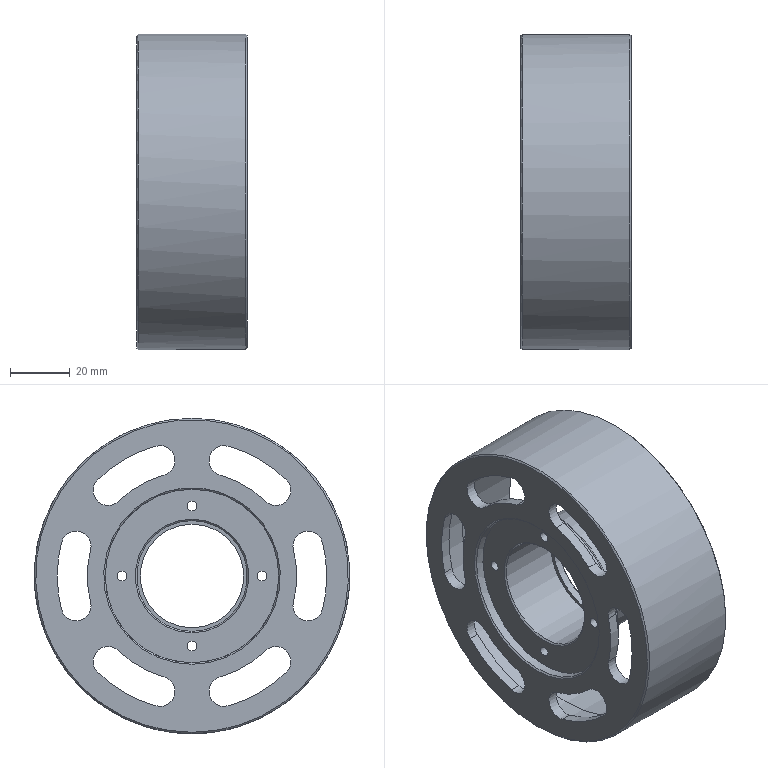Part | NX | features BREP 1 | 1 solid | 54 faces | box 37 x 105.4 x 105.4 mm | volume 69147 mm3 | cylinder 36 | cone 8 | plane 8 | torus 2 | commonest cylinder face diameters 10 x12 70 x6 90 x6 3.3 x4 34.6 x1 37 x1
STEP:
#1=CARTESIAN_POINT('',(6.5,0.,32.));
#2=VERTEX_POINT('',#1);
#3=CARTESIAN_POINT('',(6.5,0.,0.));
#4=DIRECTION('',(-1.,0.,0.));
#5=DIRECTION('',(0.,0.,1.));
#6=AXIS2_PLACEMENT_3D('',#3,#4,#5);
#7=CIRCLE('',#6,32.);
#8=EDGE_CURVE('',#2,#2,#7,.T.);
#9=ORIENTED_EDGE('',*,*,#8,.F.);
#10=EDGE_LOOP('',(#9));
#11=FACE_BOUND('',#10,.T.);
#12=CARTESIAN_POINT('',(8.5,0.,30.));
#13=VERTEX_POINT('',#12);
#14=CARTESIAN_POINT('',(8.5,0.,0.));
#15=DIRECTION('',(1.,0.,0.));
#16=DIRECTION('',(0.,0.,1.));
#17=AXIS2_PLACEMENT_3D('',#14,#15,#16);
#18=CIRCLE('',#17,30.);
#19=EDGE_CURVE('',#13,#13,#18,.T.);
#20=ORIENTED_EDGE('',*,*,#19,.F.);
#21=EDGE_LOOP('',(#20));
#22=FACE_BOUND('',#21,.T.);
#23=CARTESIAN_POINT('',(6.5,0.,0.));
#24=DIRECTION('',(-1.,0.,0.));
#25=DIRECTION('',(0.,0.,1.));
#26=AXIS2_PLACEMENT_3D('',#23,#24,#25);
#27=CONICAL_SURFACE('',#26,32.,0.7854);
#28=ADVANCED_FACE('',(#11,#22),#27,.T.);
#29=CARTESIAN_POINT('',(3.5,9.367,33.723));
#30=VERTEX_POINT('',#29);
#31=CARTESIAN_POINT('',(3.5,12.043,43.359));
#32=VERTEX_POINT('',#31);
#33=CARTESIAN_POINT('',(3.5,10.705,38.541));
#34=DIRECTION('',(-1.,0.,0.));
#35=DIRECTION('',(0.,0.,1.));
#36=AXIS2_PLACEMENT_3D('',#33,#34,#35);
#37=CIRCLE('',#36,5.);
#38=EDGE_CURVE('',#30,#32,#37,.T.);
#39=ORIENTED_EDGE('',*,*,#38,.F.);
#40=CARTESIAN_POINT('',(0.,9.367,33.723));
#41=VERTEX_POINT('',#40);
#42=CARTESIAN_POINT('',(10.,9.367,33.723));
#43=DIRECTION('',(-1.,0.,0.));
#44=VECTOR('',#43,1000.);
#45=LINE('',#42,#44);
#46=EDGE_CURVE('',#30,#41,#45,.T.);
#47=ORIENTED_EDGE('',*,*,#46,.T.);
#48=CARTESIAN_POINT('',(0.,12.043,43.359));
#49=VERTEX_POINT('',#48);
#50=CARTESIAN_POINT('',(0.,10.705,38.541));
#51=DIRECTION('',(-1.,0.,0.));
#52=DIRECTION('',(0.,-0.866,0.5));
#53=AXIS2_PLACEMENT_3D('',#50,#51,#52);
#54=CIRCLE('',#53,5.);
#55=EDGE_CURVE('',#41,#49,#54,.T.);
#56=ORIENTED_EDGE('',*,*,#55,.T.);
#57=CARTESIAN_POINT('',(10.,12.043,43.359));
#58=DIRECTION('',(-1.,0.,0.));
#59=VECTOR('',#58,1000.);
#60=LINE('',#57,#59);
#61=EDGE_CURVE('',#32,#49,#60,.T.);
#62=ORIENTED_EDGE('',*,*,#61,.F.);
#63=EDGE_LOOP('',(#39,#47,#56,#62));
#64=FACE_BOUND('',#63,.T.);
#65=CARTESIAN_POINT('',(10.,10.705,38.541));
#66=DIRECTION('',(-1.,0.,0.));
#67=DIRECTION('',(0.,0.,1.));
#68=AXIS2_PLACEMENT_3D('',#65,#66,#67);
#69=CYLINDRICAL_SURFACE('',#68,5.);
#70=ADVANCED_FACE('',(#64),#69,.F.);
#71=CARTESIAN_POINT('',(3.5,-12.043,43.359));
#72=VERTEX_POINT('',#71);
#73=CARTESIAN_POINT('',(3.5,-9.367,33.723));
#74=VERTEX_POINT('',#73);
#75=CARTESIAN_POINT('',(3.5,-10.705,38.541));
#76=DIRECTION('',(-1.,0.,0.));
#77=DIRECTION('',(0.,0.,1.));
#78=AXIS2_PLACEMENT_3D('',#75,#76,#77);
#79=CIRCLE('',#78,5.);
#80=EDGE_CURVE('',#72,#74,#79,.T.);
#81=ORIENTED_EDGE('',*,*,#80,.F.);
#82=CARTESIAN_POINT('',(0.,-12.043,43.359));
#83=VERTEX_POINT('',#82);
#84=CARTESIAN_POINT('',(10.,-12.043,43.359));
#85=DIRECTION('',(-1.,0.,0.));
#86=VECTOR('',#85,1000.);
#87=LINE('',#84,#86);
#88=EDGE_CURVE('',#72,#83,#87,.T.);
#89=ORIENTED_EDGE('',*,*,#88,.T.);
#90=CARTESIAN_POINT('',(0.,-9.367,33.723));
#91=VERTEX_POINT('',#90);
#92=CARTESIAN_POINT('',(0.,-10.705,38.541));
#93=DIRECTION('',(-1.,0.,0.));
#94=DIRECTION('',(0.,-0.866,-0.5));
#95=AXIS2_PLACEMENT_3D('',#92,#93,#94);
#96=CIRCLE('',#95,5.);
#97=EDGE_CURVE('',#83,#91,#96,.T.);
#98=ORIENTED_EDGE('',*,*,#97,.T.);
#99=CARTESIAN_POINT('',(10.,-9.367,33.723));
#100=DIRECTION('',(-1.,0.,0.));
#101=VECTOR('',#100,1000.);
#102=LINE('',#99,#101);
#103=EDGE_CURVE('',#74,#91,#102,.T.);
#104=ORIENTED_EDGE('',*,*,#103,.F.);
#105=EDGE_LOOP('',(#81,#89,#98,#104));
#106=FACE_BOUND('',#105,.T.);
#107=CARTESIAN_POINT('',(10.,-10.705,38.541));
#108=DIRECTION('',(-1.,0.,0.));
#109=DIRECTION('',(0.,0.,1.));
#110=AXIS2_PLACEMENT_3D('',#107,#108,#109);
#111=CYLINDRICAL_SURFACE('',#110,5.);
#112=ADVANCED_FACE('',(#106),#111,.F.);
#113=CARTESIAN_POINT('',(3.5,-43.571,11.25));
#114=VERTEX_POINT('',#113);
#115=CARTESIAN_POINT('',(3.5,-33.889,8.75));
#116=VERTEX_POINT('',#115);
#117=CARTESIAN_POINT('',(3.5,-38.73,10.));
#118=DIRECTION('',(-1.,0.,0.));
#119=DIRECTION('',(0.,0.,1.));
#120=AXIS2_PLACEMENT_3D('',#117,#118,#119);
#121=CIRCLE('',#120,5.);
#122=EDGE_CURVE('',#114,#116,#121,.T.);
#123=ORIENTED_EDGE('',*,*,#122,.F.);
#124=CARTESIAN_POINT('',(0.,-43.571,11.25));
#125=VERTEX_POINT('',#124);
#126=CARTESIAN_POINT('',(10.,-43.571,11.25));
#127=DIRECTION('',(-1.,0.,0.));
#128=VECTOR('',#127,1000.);
#129=LINE('',#126,#128);
#130=EDGE_CURVE('',#114,#125,#129,.T.);
#131=ORIENTED_EDGE('',*,*,#130,.T.);
#132=CARTESIAN_POINT('',(0.,-33.889,8.75));
#133=VERTEX_POINT('',#132);
#134=CARTESIAN_POINT('',(0.,-38.73,10.));
#135=DIRECTION('',(-1.,0.,0.));
#136=DIRECTION('',(0.,0.,-1.));
#137=AXIS2_PLACEMENT_3D('',#134,#135,#136);
#138=CIRCLE('',#137,5.);
#139=EDGE_CURVE('',#125,#133,#138,.T.);
#140=ORIENTED_EDGE('',*,*,#139,.T.);
#141=CARTESIAN_POINT('',(10.,-33.889,8.75));
#142=DIRECTION('',(-1.,0.,0.));
#143=VECTOR('',#142,1000.);
#144=LINE('',#141,#143);
#145=EDGE_CURVE('',#116,#133,#144,.T.);
#146=ORIENTED_EDGE('',*,*,#145,.F.);
#147=EDGE_LOOP('',(#123,#131,#140,#146));
#148=FACE_BOUND('',#147,.T.);
#149=CARTESIAN_POINT('',(10.,-38.73,10.));
#150=DIRECTION('',(-1.,0.,0.));
#151=DIRECTION('',(0.,0.,1.));
#152=AXIS2_PLACEMENT_3D('',#149,#150,#151);
#153=CYLINDRICAL_SURFACE('',#152,5.);
#154=ADVANCED_FACE('',(#148),#153,.F.);
#155=CARTESIAN_POINT('',(3.5,-31.528,-32.109));
#156=VERTEX_POINT('',#155);
#157=CARTESIAN_POINT('',(3.5,-24.522,-24.973));
#158=VERTEX_POINT('',#157);
#159=CARTESIAN_POINT('',(3.5,-28.025,-28.541));
#160=DIRECTION('',(-1.,0.,0.));
#161=DIRECTION('',(0.,0.,1.));
#162=AXIS2_PLACEMENT_3D('',#159,#160,#161);
#163=CIRCLE('',#162,5.);
#164=EDGE_CURVE('',#156,#158,#163,.T.);
#165=ORIENTED_EDGE('',*,*,#164,.F.);
#166=CARTESIAN_POINT('',(0.,-31.528,-32.109));
#167=VERTEX_POINT('',#166);
#168=CARTESIAN_POINT('',(10.,-31.528,-32.109));
#169=DIRECTION('',(-1.,0.,0.));
#170=VECTOR('',#169,1000.);
#171=LINE('',#168,#170);
#172=EDGE_CURVE('',#156,#167,#171,.T.);
#173=ORIENTED_EDGE('',*,*,#172,.T.);
#174=CARTESIAN_POINT('',(0.,-24.522,-24.973));
#175=VERTEX_POINT('',#174);
#176=CARTESIAN_POINT('',(0.,-28.025,-28.541));
#177=DIRECTION('',(-1.,0.,0.));
#178=DIRECTION('',(0.,0.866,-0.5));
#179=AXIS2_PLACEMENT_3D('',#176,#177,#178);
#180=CIRCLE('',#179,5.);
#181=EDGE_CURVE('',#167,#175,#180,.T.);
#182=ORIENTED_EDGE('',*,*,#181,.T.);
#183=CARTESIAN_POINT('',(10.,-24.522,-24.973));
#184=DIRECTION('',(-1.,0.,0.));
#185=VECTOR('',#184,1000.);
#186=LINE('',#183,#185);
#187=EDGE_CURVE('',#158,#175,#186,.T.);
#188=ORIENTED_EDGE('',*,*,#187,.F.);
#189=EDGE_LOOP('',(#165,#173,#182,#188));
#190=FACE_BOUND('',#189,.T.);
#191=CARTESIAN_POINT('',(10.,-28.025,-28.541));
#192=DIRECTION('',(-1.,0.,0.));
#193=DIRECTION('',(0.,0.,1.));
#194=AXIS2_PLACEMENT_3D('',#191,#192,#193);
#195=CYLINDRICAL_SURFACE('',#194,5.);
#196=ADVANCED_FACE('',(#190),#195,.F.);
#197=CARTESIAN_POINT('',(3.5,24.522,-24.973));
#198=VERTEX_POINT('',#197);
#199=CARTESIAN_POINT('',(3.5,31.528,-32.109));
#200=VERTEX_POINT('',#199);
#201=CARTESIAN_POINT('',(3.5,28.025,-28.541));
#202=DIRECTION('',(-1.,0.,0.));
#203=DIRECTION('',(0.,0.,1.));
#204=AXIS2_PLACEMENT_3D('',#201,#202,#203);
#205=CIRCLE('',#204,5.);
#206=EDGE_CURVE('',#198,#200,#205,.T.);
#207=ORIENTED_EDGE('',*,*,#206,.F.);
#208=CARTESIAN_POINT('',(0.,24.522,-24.973));
#209=VERTEX_POINT('',#208);
#210=CARTESIAN_POINT('',(10.,24.522,-24.973));
#211=DIRECTION('',(-1.,0.,0.));
#212=VECTOR('',#211,1000.);
#213=LINE('',#210,#212);
#214=EDGE_CURVE('',#198,#209,#213,.T.);
#215=ORIENTED_EDGE('',*,*,#214,.T.);
#216=CARTESIAN_POINT('',(0.,31.528,-32.109));
#217=VERTEX_POINT('',#216);
#218=CARTESIAN_POINT('',(0.,28.025,-28.541));
#219=DIRECTION('',(-1.,0.,0.));
#220=DIRECTION('',(0.,0.866,0.5));
#221=AXIS2_PLACEMENT_3D('',#218,#219,#220);
#222=CIRCLE('',#221,5.);
#223=EDGE_CURVE('',#209,#217,#222,.T.);
#224=ORIENTED_EDGE('',*,*,#223,.T.);
#225=CARTESIAN_POINT('',(10.,31.528,-32.109));
#226=DIRECTION('',(-1.,0.,0.));
#227=VECTOR('',#226,1000.);
#228=LINE('',#225,#227);
#229=EDGE_CURVE('',#200,#217,#228,.T.);
#230=ORIENTED_EDGE('',*,*,#229,.F.);
#231=EDGE_LOOP('',(#207,#215,#224,#230));
#232=FACE_BOUND('',#231,.T.);
#233=CARTESIAN_POINT('',(10.,28.025,-28.541));
#234=DIRECTION('',(-1.,0.,0.));
#235=DIRECTION('',(0.,0.,1.));
#236=AXIS2_PLACEMENT_3D('',#233,#234,#235);
#237=CYLINDRICAL_SURFACE('',#236,5.);
#238=ADVANCED_FACE('',(#232),#237,.F.);
#239=CARTESIAN_POINT('',(3.5,33.889,8.75));
#240=VERTEX_POINT('',#239);
#241=CARTESIAN_POINT('',(3.5,43.571,11.25));
#242=VERTEX_POINT('',#241);
#243=CARTESIAN_POINT('',(3.5,38.73,10.));
#244=DIRECTION('',(-1.,0.,0.));
#245=DIRECTION('',(0.,0.,1.));
#246=AXIS2_PLACEMENT_3D('',#243,#244,#245);
#247=CIRCLE('',#246,5.);
#248=EDGE_CURVE('',#240,#242,#247,.T.);
#249=ORIENTED_EDGE('',*,*,#248,.F.);
#250=CARTESIAN_POINT('',(0.,33.889,8.75));
#251=VERTEX_POINT('',#250);
#252=CARTESIAN_POINT('',(10.,33.889,8.75));
#253=DIRECTION('',(-1.,0.,0.));
#254=VECTOR('',#253,1000.);
#255=LINE('',#252,#254);
#256=EDGE_CURVE('',#240,#251,#255,.T.);
#257=ORIENTED_EDGE('',*,*,#256,.T.);
#258=CARTESIAN_POINT('',(0.,43.571,11.25));
#259=VERTEX_POINT('',#258);
#260=CARTESIAN_POINT('',(0.,38.73,10.));
#261=DIRECTION('',(-1.,0.,0.));
#262=DIRECTION('',(0.,0.,1.));
#263=AXIS2_PLACEMENT_3D('',#260,#261,#262);
#264=CIRCLE('',#263,5.);
#265=EDGE_CURVE('',#251,#259,#264,.T.);
#266=ORIENTED_EDGE('',*,*,#265,.T.);
#267=CARTESIAN_POINT('',(10.,43.571,11.25));
#268=DIRECTION('',(-1.,0.,0.));
#269=VECTOR('',#268,1000.);
#270=LINE('',#267,#269);
#271=EDGE_CURVE('',#242,#259,#270,.T.);
#272=ORIENTED_EDGE('',*,*,#271,.F.);
#273=EDGE_LOOP('',(#249,#257,#266,#272));
#274=FACE_BOUND('',#273,.T.);
#275=CARTESIAN_POINT('',(10.,38.73,10.));
#276=DIRECTION('',(-1.,0.,0.));
#277=DIRECTION('',(0.,0.,1.));
#278=AXIS2_PLACEMENT_3D('',#275,#276,#277);
#279=CYLINDRICAL_SURFACE('',#278,5.);
#280=ADVANCED_FACE('',(#274),#279,.F.);
#281=CARTESIAN_POINT('',(3.5,23.4,1.65));
#282=VERTEX_POINT('',#281);
#283=CARTESIAN_POINT('',(3.5,23.4,0.));
#284=DIRECTION('',(-1.,0.,0.));
#285=DIRECTION('',(0.,0.,1.));
#286=AXIS2_PLACEMENT_3D('',#283,#284,#285);
#287=CIRCLE('',#286,1.65);
#288=EDGE_CURVE('',#282,#282,#287,.T.);
#289=ORIENTED_EDGE('',*,*,#288,.T.);
#290=EDGE_LOOP('',(#289));
#291=FACE_BOUND('',#290,.T.);
#292=CARTESIAN_POINT('',(8.5,23.4,1.65));
#293=VERTEX_POINT('',#292);
#294=CARTESIAN_POINT('',(8.5,23.4,0.));
#295=DIRECTION('',(-1.,0.,0.));
#296=DIRECTION('',(0.,0.,1.));
#297=AXIS2_PLACEMENT_3D('',#294,#295,#296);
#298=CIRCLE('',#297,1.65);
#299=EDGE_CURVE('',#293,#293,#298,.T.);
#300=ORIENTED_EDGE('',*,*,#299,.F.);
#301=EDGE_LOOP('',(#300));
#302=FACE_BOUND('',#301,.T.);
#303=CARTESIAN_POINT('',(3.5,23.4,0.));
#304=DIRECTION('',(-1.,0.,0.));
#305=DIRECTION('',(0.,0.,1.));
#306=AXIS2_PLACEMENT_3D('',#303,#304,#305);
#307=CYLINDRICAL_SURFACE('',#306,1.65);
#308=ADVANCED_FACE('',(#291,#302),#307,.F.);
#309=CARTESIAN_POINT('',(3.5,0.,25.05));
#310=VERTEX_POINT('',#309);
#311=CARTESIAN_POINT('',(3.5,0.,23.4));
#312=DIRECTION('',(-1.,0.,0.));
#313=DIRECTION('',(0.,0.,1.));
#314=AXIS2_PLACEMENT_3D('',#311,#312,#313);
#315=CIRCLE('',#314,1.65);
#316=EDGE_CURVE('',#310,#310,#315,.T.);
#317=ORIENTED_EDGE('',*,*,#316,.T.);
#318=EDGE_LOOP('',(#317));
#319=FACE_BOUND('',#318,.T.);
#320=CARTESIAN_POINT('',(8.5,0.,25.05));
#321=VERTEX_POINT('',#320);
#322=CARTESIAN_POINT('',(8.5,0.,23.4));
#323=DIRECTION('',(-1.,0.,0.));
#324=DIRECTION('',(0.,0.,1.));
#325=AXIS2_PLACEMENT_3D('',#322,#323,#324);
#326=CIRCLE('',#325,1.65);
#327=EDGE_CURVE('',#321,#321,#326,.T.);
#328=ORIENTED_EDGE('',*,*,#327,.F.);
#329=EDGE_LOOP('',(#328));
#330=FACE_BOUND('',#329,.T.);
#331=CARTESIAN_POINT('',(3.5,0.,23.4));
#332=DIRECTION('',(-1.,0.,0.));
#333=DIRECTION('',(0.,0.,1.));
#334=AXIS2_PLACEMENT_3D('',#331,#332,#333);
#335=CYLINDRICAL_SURFACE('',#334,1.65);
#336=ADVANCED_FACE('',(#319,#330),#335,.F.);
#337=CARTESIAN_POINT('',(3.5,-23.4,1.65));
#338=VERTEX_POINT('',#337);
#339=CARTESIAN_POINT('',(3.5,-23.4,0.));
#340=DIRECTION('',(-1.,0.,0.));
#341=DIRECTION('',(0.,0.,1.));
#342=AXIS2_PLACEMENT_3D('',#339,#340,#341);
#343=CIRCLE('',#342,1.65);
#344=EDGE_CURVE('',#338,#338,#343,.T.);
#345=ORIENTED_EDGE('',*,*,#344,.T.);
#346=EDGE_LOOP('',(#345));
#347=FACE_BOUND('',#346,.T.);
#348=CARTESIAN_POINT('',(8.5,-23.4,1.65));
#349=VERTEX_POINT('',#348);
#350=CARTESIAN_POINT('',(8.5,-23.4,0.));
#351=DIRECTION('',(-1.,0.,0.));
#352=DIRECTION('',(0.,0.,1.));
#353=AXIS2_PLACEMENT_3D('',#350,#351,#352);
#354=CIRCLE('',#353,1.65);
#355=EDGE_CURVE('',#349,#349,#354,.T.);
#356=ORIENTED_EDGE('',*,*,#355,.F.);
#357=EDGE_LOOP('',(#356));
#358=FACE_BOUND('',#357,.T.);
#359=CARTESIAN_POINT('',(3.5,-23.4,0.));
#360=DIRECTION('',(-1.,0.,0.));
#361=DIRECTION('',(0.,0.,1.));
#362=AXIS2_PLACEMENT_3D('',#359,#360,#361);
#363=CYLINDRICAL_SURFACE('',#362,1.65);
#364=ADVANCED_FACE('',(#347,#358),#363,.F.);
#365=CARTESIAN_POINT('',(3.5,0.,-21.75));
#366=VERTEX_POINT('',#365);
#367=CARTESIAN_POINT('',(3.5,0.,-23.4));
#368=DIRECTION('',(-1.,0.,0.));
#369=DIRECTION('',(0.,0.,1.));
#370=AXIS2_PLACEMENT_3D('',#367,#368,#369);
#371=CIRCLE('',#370,1.65);
#372=EDGE_CURVE('',#366,#366,#371,.T.);
#373=ORIENTED_EDGE('',*,*,#372,.T.);
#374=EDGE_LOOP('',(#373));
#375=FACE_BOUND('',#374,.T.);
#376=CARTESIAN_POINT('',(8.5,0.,-21.75));
#377=VERTEX_POINT('',#376);
#378=CARTESIAN_POINT('',(8.5,0.,-23.4));
#379=DIRECTION('',(-1.,0.,0.));
#380=DIRECTION('',(0.,0.,1.));
#381=AXIS2_PLACEMENT_3D('',#378,#379,#380);
#382=CIRCLE('',#381,1.65);
#383=EDGE_CURVE('',#377,#377,#382,.T.);
#384=ORIENTED_EDGE('',*,*,#383,.F.);
#385=EDGE_LOOP('',(#384));
#386=FACE_BOUND('',#385,.T.);
#387=CARTESIAN_POINT('',(3.5,0.,-23.4));
#388=DIRECTION('',(-1.,0.,0.));
#389=DIRECTION('',(0.,0.,1.));
#390=AXIS2_PLACEMENT_3D('',#387,#388,#389);
#391=CYLINDRICAL_SURFACE('',#390,1.65);
#392=ADVANCED_FACE('',(#375,#386),#391,.F.);
#393=CARTESIAN_POINT('',(28.,0.,17.8));
#394=VERTEX_POINT('',#393);
#395=CARTESIAN_POINT('',(28.,0.,0.));
#396=DIRECTION('',(-1.,0.,0.));
#397=DIRECTION('',(0.,0.,1.));
#398=AXIS2_PLACEMENT_3D('',#395,#396,#397);
#399=CIRCLE('',#398,17.8);
#400=EDGE_CURVE('',#394,#394,#399,.T.);
#401=ORIENTED_EDGE('',*,*,#400,.F.);
#402=EDGE_LOOP('',(#401));
#403=FACE_BOUND('',#402,.T.);
#404=CARTESIAN_POINT('',(27.5,0.,17.3));
#405=VERTEX_POINT('',#404);
#406=CARTESIAN_POINT('',(27.5,0.,0.));
#407=DIRECTION('',(1.,0.,0.));
#408=DIRECTION('',(0.,0.,1.));
#409=AXIS2_PLACEMENT_3D('',#406,#407,#408);
#410=CIRCLE('',#409,17.3);
#411=EDGE_CURVE('',#405,#405,#410,.T.);
#412=ORIENTED_EDGE('',*,*,#411,.F.);
#413=EDGE_LOOP('',(#412));
#414=FACE_BOUND('',#413,.T.);
#415=CARTESIAN_POINT('',(28.,0.,0.));
#416=DIRECTION('',(1.,0.,0.));
#417=DIRECTION('',(0.,0.,-1.));
#418=AXIS2_PLACEMENT_3D('',#415,#416,#417);
#419=CONICAL_SURFACE('',#418,17.8,0.7854);
#420=ADVANCED_FACE('',(#403,#414),#419,.F.);
#421=CARTESIAN_POINT('',(0.5,0.,-52.7));
#422=VERTEX_POINT('',#421);
#423=CARTESIAN_POINT('',(0.5,0.,0.));
#424=DIRECTION('',(1.,0.,0.));
#425=DIRECTION('',(0.,0.,-1.));
#426=AXIS2_PLACEMENT_3D('',#423,#424,#425);
#427=CIRCLE('',#426,52.7);
#428=EDGE_CURVE('',#422,#422,#427,.T.);
#429=ORIENTED_EDGE('',*,*,#428,.F.);
#430=EDGE_LOOP('',(#429));
#431=FACE_BOUND('',#430,.T.);
#432=CARTESIAN_POINT('',(0.,0.,-52.2));
#433=VERTEX_POINT('',#432);
#434=CARTESIAN_POINT('',(0.,0.,0.));
#435=DIRECTION('',(-1.,0.,0.));
#436=DIRECTION('',(0.,0.,-1.));
#437=AXIS2_PLACEMENT_3D('',#434,#435,#436);
#438=CIRCLE('',#437,52.2);
#439=EDGE_CURVE('',#433,#433,#438,.T.);
#440=ORIENTED_EDGE('',*,*,#439,.F.);
#441=EDGE_LOOP('',(#440));
#442=FACE_BOUND('',#441,.T.);
#443=CARTESIAN_POINT('',(0.,0.,0.));
#444=DIRECTION('',(1.,0.,0.));
#445=DIRECTION('',(0.,0.,-1.));
#446=AXIS2_PLACEMENT_3D('',#443,#444,#445);
#447=CONICAL_SURFACE('',#446,52.2,0.7854);
#448=ADVANCED_FACE('',(#431,#442),#447,.T.);
#449=CARTESIAN_POINT('',(0.,0.,-29.5));
#450=VERTEX_POINT('',#449);
#451=CARTESIAN_POINT('',(0.,0.,0.));
#452=DIRECTION('',(1.,0.,0.));
#453=DIRECTION('',(0.,0.,-1.));
#454=AXIS2_PLACEMENT_3D('',#451,#452,#453);
#455=CIRCLE('',#454,29.5);
#456=EDGE_CURVE('',#450,#450,#455,.T.);
#457=ORIENTED_EDGE('',*,*,#456,.F.);
#458=EDGE_LOOP('',(#457));
#459=FACE_BOUND('',#458,.T.);
#460=CARTESIAN_POINT('',(0.5,0.,-29.));
#461=VERTEX_POINT('',#460);
#462=CARTESIAN_POINT('',(0.5,0.,0.));
#463=DIRECTION('',(-1.,0.,0.));
#464=DIRECTION('',(0.,0.,-1.));
#465=AXIS2_PLACEMENT_3D('',#462,#463,#464);
#466=CIRCLE('',#465,29.);
#467=EDGE_CURVE('',#461,#461,#466,.T.);
#468=ORIENTED_EDGE('',*,*,#467,.F.);
#469=EDGE_LOOP('',(#468));
#470=FACE_BOUND('',#469,.T.);
#471=CARTESIAN_POINT('',(0.5,0.,0.));
#472=DIRECTION('',(-1.,0.,0.));
#473=DIRECTION('',(0.,0.,1.));
#474=AXIS2_PLACEMENT_3D('',#471,#472,#473);
#475=CONICAL_SURFACE('',#474,29.,0.7854);
#476=ADVANCED_FACE('',(#459,#470),#475,.F.);
#477=CARTESIAN_POINT('',(3.5,0.,-19.));
#478=VERTEX_POINT('',#477);
#479=CARTESIAN_POINT('',(3.5,0.,0.));
#480=DIRECTION('',(1.,0.,0.));
#481=DIRECTION('',(0.,0.,-1.));
#482=AXIS2_PLACEMENT_3D('',#479,#480,#481);
#483=CIRCLE('',#482,19.);
#484=EDGE_CURVE('',#478,#478,#483,.T.);
#485=ORIENTED_EDGE('',*,*,#484,.F.);
#486=EDGE_LOOP('',(#485));
#487=FACE_BOUND('',#486,.T.);
#488=CARTESIAN_POINT('',(4.,0.,-18.5));
#489=VERTEX_POINT('',#488);
#490=CARTESIAN_POINT('',(4.,0.,0.));
#491=DIRECTION('',(-1.,0.,0.));
#492=DIRECTION('',(0.,0.,-1.));
#493=AXIS2_PLACEMENT_3D('',#490,#491,#492);
#494=CIRCLE('',#493,18.5);
#495=EDGE_CURVE('',#489,#489,#494,.T.);
#496=ORIENTED_EDGE('',*,*,#495,.F.);
#497=EDGE_LOOP('',(#496));
#498=FACE_BOUND('',#497,.T.);
#499=CARTESIAN_POINT('',(4.,0.,0.));
#500=DIRECTION('',(-1.,0.,0.));
#501=DIRECTION('',(0.,0.,1.));
#502=AXIS2_PLACEMENT_3D('',#499,#500,#501);
#503=CONICAL_SURFACE('',#502,18.5,0.7854);
#504=ADVANCED_FACE('',(#487,#498),#503,.F.);
#505=CARTESIAN_POINT('',(27.5,0.,21.25));
#506=VERTEX_POINT('',#505);
#507=CARTESIAN_POINT('',(27.5,0.,0.));
#508=DIRECTION('',(-1.,0.,0.));
#509=DIRECTION('',(0.,0.,1.));
#510=AXIS2_PLACEMENT_3D('',#507,#508,#509);
#511=CIRCLE('',#510,21.25);
#512=EDGE_CURVE('',#506,#506,#511,.T.);
#513=ORIENTED_EDGE('',*,*,#512,.F.);
#514=EDGE_LOOP('',(#513));
#515=FACE_BOUND('',#514,.T.);
#516=CARTESIAN_POINT('',(28.,0.,20.75));
#517=VERTEX_POINT('',#516);
#518=CARTESIAN_POINT('',(28.,0.,0.));
#519=DIRECTION('',(1.,0.,0.));
#520=DIRECTION('',(0.,0.,1.));
#521=AXIS2_PLACEMENT_3D('',#518,#519,#520);
#522=CIRCLE('',#521,20.75);
#523=EDGE_CURVE('',#517,#517,#522,.T.);
#524=ORIENTED_EDGE('',*,*,#523,.F.);
#525=EDGE_LOOP('',(#524));
#526=FACE_BOUND('',#525,.T.);
#527=CARTESIAN_POINT('',(27.5,0.,0.));
#528=DIRECTION('',(-1.,0.,0.));
#529=DIRECTION('',(0.,0.,1.));
#530=AXIS2_PLACEMENT_3D('',#527,#528,#529);
#531=CONICAL_SURFACE('',#530,21.25,0.7854);
#532=ADVANCED_FACE('',(#515,#526),#531,.T.);
#533=CARTESIAN_POINT('',(37.,0.,49.9));
#534=VERTEX_POINT('',#533);
#535=CARTESIAN_POINT('',(37.,0.,0.));
#536=DIRECTION('',(-1.,0.,0.));
#537=DIRECTION('',(0.,0.,1.));
#538=AXIS2_PLACEMENT_3D('',#535,#536,#537);
#539=CIRCLE('',#538,49.9);
#540=EDGE_CURVE('',#534,#534,#539,.T.);
#541=ORIENTED_EDGE('',*,*,#540,.F.);
#542=EDGE_LOOP('',(#541));
#543=FACE_BOUND('',#542,.T.);
#544=CARTESIAN_POINT('',(36.5,0.,49.4));
#545=VERTEX_POINT('',#544);
#546=CARTESIAN_POINT('',(36.5,0.,0.));
#547=DIRECTION('',(1.,0.,0.));
#548=DIRECTION('',(0.,0.,1.));
#549=AXIS2_PLACEMENT_3D('',#546,#547,#548);
#550=CIRCLE('',#549,49.4);
#551=EDGE_CURVE('',#545,#545,#550,.T.);
#552=ORIENTED_EDGE('',*,*,#551,.F.);
#553=EDGE_LOOP('',(#552));
#554=FACE_BOUND('',#553,.T.);
#555=CARTESIAN_POINT('',(37.,0.,0.));
#556=DIRECTION('',(1.,0.,0.));
#557=DIRECTION('',(0.,0.,-1.));
#558=AXIS2_PLACEMENT_3D('',#555,#556,#557);
#559=CONICAL_SURFACE('',#558,49.9,0.7854);
#560=ADVANCED_FACE('',(#543,#554),#559,.F.);
#561=CARTESIAN_POINT('',(36.5,0.,52.7));
#562=VERTEX_POINT('',#561);
#563=CARTESIAN_POINT('',(36.5,0.,0.));
#564=DIRECTION('',(-1.,0.,0.));
#565=DIRECTION('',(0.,0.,1.));
#566=AXIS2_PLACEMENT_3D('',#563,#564,#565);
#567=CIRCLE('',#566,52.7);
#568=EDGE_CURVE('',#562,#562,#567,.T.);
#569=ORIENTED_EDGE('',*,*,#568,.F.);
#570=EDGE_LOOP('',(#569));
#571=FACE_BOUND('',#570,.T.);
#572=CARTESIAN_POINT('',(37.,0.,52.2));
#573=VERTEX_POINT('',#572);
#574=CARTESIAN_POINT('',(37.,0.,0.));
#575=DIRECTION('',(1.,0.,0.));
#576=DIRECTION('',(0.,0.,1.));
#577=AXIS2_PLACEMENT_3D('',#574,#575,#576);
#578=CIRCLE('',#577,52.2);
#579=EDGE_CURVE('',#573,#573,#578,.T.);
#580=ORIENTED_EDGE('',*,*,#579,.F.);
#581=EDGE_LOOP('',(#580));
#582=FACE_BOUND('',#581,.T.);
#583=CARTESIAN_POINT('',(36.5,0.,0.));
#584=DIRECTION('',(-1.,0.,0.));
#585=DIRECTION('',(0.,0.,1.));
#586=AXIS2_PLACEMENT_3D('',#583,#584,#585);
#587=CONICAL_SURFACE('',#586,52.7,0.7854);
#588=ADVANCED_FACE('',(#571,#582),#587,.T.);
#589=CARTESIAN_POINT('',(25.,0.,17.3));
#590=VERTEX_POINT('',#589);
#591=CARTESIAN_POINT('',(25.,0.,0.));
#592=DIRECTION('',(-1.,0.,0.));
#593=DIRECTION('',(0.,0.,1.));
#594=AXIS2_PLACEMENT_3D('',#591,#592,#593);
#595=CIRCLE('',#594,17.3);
#596=EDGE_CURVE('',#590,#590,#595,.T.);
#597=ORIENTED_EDGE('',*,*,#596,.T.);
#598=EDGE_LOOP('',(#597));
#599=FACE_BOUND('',#598,.T.);
#600=ORIENTED_EDGE('',*,*,#411,.T.);
#601=EDGE_LOOP('',(#600));
#602=FACE_BOUND('',#601,.T.);
#603=CARTESIAN_POINT('',(-21.345,0.,0.));
#604=DIRECTION('',(-1.,0.,0.));
#605=DIRECTION('',(0.,0.,1.));
#606=AXIS2_PLACEMENT_3D('',#603,#604,#605);
#607=CYLINDRICAL_SURFACE('',#606,17.3);
#608=ADVANCED_FACE('',(#599,#602),#607,.F.);
#609=CARTESIAN_POINT('',(8.5,0.,21.25));
#610=VERTEX_POINT('',#609);
#611=CARTESIAN_POINT('',(8.5,0.,0.));
#612=DIRECTION('',(-1.,0.,0.));
#613=DIRECTION('',(0.,0.,1.));
#614=AXIS2_PLACEMENT_3D('',#611,#612,#613);
#615=CIRCLE('',#614,21.25);
#616=EDGE_CURVE('',#610,#610,#615,.T.);
#617=ORIENTED_EDGE('',*,*,#616,.F.);
#618=EDGE_LOOP('',(#617));
#619=FACE_BOUND('',#618,.T.);
#620=ORIENTED_EDGE('',*,*,#512,.T.);
#621=EDGE_LOOP('',(#620));
#622=FACE_BOUND('',#621,.T.);
#623=CARTESIAN_POINT('',(-21.345,0.,0.));
#624=DIRECTION('',(-1.,0.,0.));
#625=DIRECTION('',(0.,0.,1.));
#626=AXIS2_PLACEMENT_3D('',#623,#624,#625);
#627=CYLINDRICAL_SURFACE('',#626,21.25);
#628=ADVANCED_FACE('',(#619,#622),#627,.T.);
#629=CARTESIAN_POINT('',(5.5,0.,32.));
#630=VERTEX_POINT('',#629);
#631=CARTESIAN_POINT('',(5.5,0.,0.));
#632=DIRECTION('',(-1.,0.,0.));
#633=DIRECTION('',(0.,0.,1.));
#634=AXIS2_PLACEMENT_3D('',#631,#632,#633);
#635=CIRCLE('',#634,32.);
#636=EDGE_CURVE('',#630,#630,#635,.T.);
#637=ORIENTED_EDGE('',*,*,#636,.F.);
#638=EDGE_LOOP('',(#637));
#639=FACE_BOUND('',#638,.T.);
#640=ORIENTED_EDGE('',*,*,#8,.T.);
#641=EDGE_LOOP('',(#640));
#642=FACE_BOUND('',#641,.T.);
#643=CARTESIAN_POINT('',(-21.345,0.,0.));
#644=DIRECTION('',(-1.,0.,0.));
#645=DIRECTION('',(0.,0.,1.));
#646=AXIS2_PLACEMENT_3D('',#643,#644,#645);
#647=CYLINDRICAL_SURFACE('',#646,32.);
#648=ADVANCED_FACE('',(#639,#642),#647,.T.);
#649=ORIENTED_EDGE('',*,*,#636,.T.);
#650=EDGE_LOOP('',(#649));
#651=FACE_BOUND('',#650,.T.);
#652=CARTESIAN_POINT('',(3.5,0.,34.));
#653=VERTEX_POINT('',#652);
#654=CARTESIAN_POINT('',(3.5,0.,0.));
#655=DIRECTION('',(-1.,0.,0.));
#656=DIRECTION('',(0.,0.,1.));
#657=AXIS2_PLACEMENT_3D('',#654,#655,#656);
#658=CIRCLE('',#657,34.);
#659=EDGE_CURVE('',#653,#653,#658,.T.);
#660=ORIENTED_EDGE('',*,*,#659,.F.);
#661=EDGE_LOOP('',(#660));
#662=FACE_BOUND('',#661,.T.);
#663=CARTESIAN_POINT('',(5.5,0.,0.));
#664=DIRECTION('',(-1.,0.,0.));
#665=DIRECTION('',(0.,0.,1.));
#666=AXIS2_PLACEMENT_3D('',#663,#664,#665);
#667=TOROIDAL_SURFACE('',#666,34.,2.);
#668=ADVANCED_FACE('',(#651,#662),#667,.F.);
#669=CARTESIAN_POINT('',(3.5,0.,47.15));
#670=VERTEX_POINT('',#669);
#671=CARTESIAN_POINT('',(3.5,0.,0.));
#672=DIRECTION('',(-1.,0.,0.));
#673=DIRECTION('',(0.,0.,1.));
#674=AXIS2_PLACEMENT_3D('',#671,#672,#673);
#675=CIRCLE('',#674,47.15);
#676=EDGE_CURVE('',#670,#670,#675,.T.);
#677=ORIENTED_EDGE('',*,*,#676,.T.);
#678=EDGE_LOOP('',(#677));
#679=FACE_BOUND('',#678,.T.);
#680=CARTESIAN_POINT('',(5.5,0.,49.15));
#681=VERTEX_POINT('',#680);
#682=CARTESIAN_POINT('',(5.5,0.,0.));
#683=DIRECTION('',(-1.,0.,0.));
#684=DIRECTION('',(0.,0.,1.));
#685=AXIS2_PLACEMENT_3D('',#682,#683,#684);
#686=CIRCLE('',#685,49.15);
#687=EDGE_CURVE('',#681,#681,#686,.T.);
#688=ORIENTED_EDGE('',*,*,#687,.F.);
#689=EDGE_LOOP('',(#688));
#690=FACE_BOUND('',#689,.T.);
#691=CARTESIAN_POINT('',(5.5,0.,0.));
#692=DIRECTION('',(-1.,0.,0.));
#693=DIRECTION('',(0.,0.,1.));
#694=AXIS2_PLACEMENT_3D('',#691,#692,#693);
#695=TOROIDAL_SURFACE('',#694,47.15,2.);
#696=ADVANCED_FACE('',(#679,#690),#695,.F.);
#697=ORIENTED_EDGE('',*,*,#687,.T.);
#698=EDGE_LOOP('',(#697));
#699=FACE_BOUND('',#698,.T.);
#700=CARTESIAN_POINT('',(13.8,0.,49.15));
#701=VERTEX_POINT('',#700);
#702=CARTESIAN_POINT('',(13.8,0.,0.));
#703=DIRECTION('',(-1.,0.,0.));
#704=DIRECTION('',(0.,0.,1.));
#705=AXIS2_PLACEMENT_3D('',#702,#703,#704);
#706=CIRCLE('',#705,49.15);
#707=EDGE_CURVE('',#701,#701,#706,.T.);
#708=ORIENTED_EDGE('',*,*,#707,.F.);
#709=EDGE_LOOP('',(#708));
#710=FACE_BOUND('',#709,.T.);
#711=CARTESIAN_POINT('',(-21.345,0.,0.));
#712=DIRECTION('',(-1.,0.,0.));
#713=DIRECTION('',(0.,0.,1.));
#714=AXIS2_PLACEMENT_3D('',#711,#712,#713);
#715=CYLINDRICAL_SURFACE('',#714,49.15);
#716=ADVANCED_FACE('',(#699,#710),#715,.F.);
#717=CARTESIAN_POINT('',(13.8,0.,49.4));
#718=VERTEX_POINT('',#717);
#719=CARTESIAN_POINT('',(13.8,0.,0.));
#720=DIRECTION('',(-1.,0.,0.));
#721=DIRECTION('',(0.,0.,1.));
#722=AXIS2_PLACEMENT_3D('',#719,#720,#721);
#723=CIRCLE('',#722,49.4);
#724=EDGE_CURVE('',#718,#718,#723,.T.);
#725=ORIENTED_EDGE('',*,*,#724,.T.);
#726=EDGE_LOOP('',(#725));
#727=FACE_BOUND('',#726,.T.);
#728=ORIENTED_EDGE('',*,*,#551,.T.);
#729=EDGE_LOOP('',(#728));
#730=FACE_BOUND('',#729,.T.);
#731=CARTESIAN_POINT('',(-21.345,0.,0.));
#732=DIRECTION('',(-1.,0.,0.));
#733=DIRECTION('',(0.,0.,1.));
#734=AXIS2_PLACEMENT_3D('',#731,#732,#733);
#735=CYLINDRICAL_SURFACE('',#734,49.4);
#736=ADVANCED_FACE('',(#727,#730),#735,.F.);
#737=ORIENTED_EDGE('',*,*,#428,.T.);
#738=EDGE_LOOP('',(#737));
#739=FACE_BOUND('',#738,.T.);
#740=ORIENTED_EDGE('',*,*,#568,.T.);
#741=EDGE_LOOP('',(#740));
#742=FACE_BOUND('',#741,.T.);
#743=CARTESIAN_POINT('',(-21.345,0.,0.));
#744=DIRECTION('',(-1.,0.,0.));
#745=DIRECTION('',(0.,0.,1.));
#746=AXIS2_PLACEMENT_3D('',#743,#744,#745);
#747=CYLINDRICAL_SURFACE('',#746,52.7);
#748=ADVANCED_FACE('',(#739,#742),#747,.T.);
#749=ORIENTED_EDGE('',*,*,#467,.T.);
#750=EDGE_LOOP('',(#749));
#751=FACE_BOUND('',#750,.T.);
#752=CARTESIAN_POINT('',(3.5,0.,29.));
#753=VERTEX_POINT('',#752);
#754=CARTESIAN_POINT('',(3.5,0.,0.));
#755=DIRECTION('',(-1.,0.,0.));
#756=DIRECTION('',(0.,0.,1.));
#757=AXIS2_PLACEMENT_3D('',#754,#755,#756);
#758=CIRCLE('',#757,29.);
#759=EDGE_CURVE('',#753,#753,#758,.T.);
#760=ORIENTED_EDGE('',*,*,#759,.F.);
#761=EDGE_LOOP('',(#760));
#762=FACE_BOUND('',#761,.T.);
#763=CARTESIAN_POINT('',(-21.345,0.,0.));
#764=DIRECTION('',(-1.,0.,0.));
#765=DIRECTION('',(0.,0.,1.));
#766=AXIS2_PLACEMENT_3D('',#763,#764,#765);
#767=CYLINDRICAL_SURFACE('',#766,29.);
#768=ADVANCED_FACE('',(#751,#762),#767,.F.);
#769=ORIENTED_EDGE('',*,*,#495,.T.);
#770=EDGE_LOOP('',(#769));
#771=FACE_BOUND('',#770,.T.);
#772=CARTESIAN_POINT('',(25.,0.,18.5));
#773=VERTEX_POINT('',#772);
#774=CARTESIAN_POINT('',(25.,0.,0.));
#775=DIRECTION('',(-1.,0.,0.));
#776=DIRECTION('',(0.,0.,1.));
#777=AXIS2_PLACEMENT_3D('',#774,#775,#776);
#778=CIRCLE('',#777,18.5);
#779=EDGE_CURVE('',#773,#773,#778,.T.);
#780=ORIENTED_EDGE('',*,*,#779,.F.);
#781=EDGE_LOOP('',(#780));
#782=FACE_BOUND('',#781,.T.);
#783=CARTESIAN_POINT('',(-21.345,0.,0.));
#784=DIRECTION('',(-1.,0.,0.));
#785=DIRECTION('',(0.,0.,1.));
#786=AXIS2_PLACEMENT_3D('',#783,#784,#785);
#787=CYLINDRICAL_SURFACE('',#786,18.5);
#788=ADVANCED_FACE('',(#771,#782),#787,.F.);
#789=ORIENTED_EDGE('',*,*,#596,.F.);
#790=EDGE_LOOP('',(#789));
#791=FACE_BOUND('',#790,.T.);
#792=ORIENTED_EDGE('',*,*,#779,.T.);
#793=EDGE_LOOP('',(#792));
#794=FACE_BOUND('',#793,.T.);
#795=CARTESIAN_POINT('',(25.,18.5,0.));
#796=DIRECTION('',(1.,0.,0.));
#797=DIRECTION('',(0.,0.,-1.));
#798=AXIS2_PLACEMENT_3D('',#795,#796,#797);
#799=PLANE('',#798);
#800=ADVANCED_FACE('',(#791,#794),#799,.F.);
#801=ORIENTED_EDGE('',*,*,#288,.F.);
#802=EDGE_LOOP('',(#801));
#803=FACE_BOUND('',#802,.T.);
#804=ORIENTED_EDGE('',*,*,#316,.F.);
#805=EDGE_LOOP('',(#804));
#806=FACE_BOUND('',#805,.T.);
#807=ORIENTED_EDGE('',*,*,#344,.F.);
#808=EDGE_LOOP('',(#807));
#809=FACE_BOUND('',#808,.T.);
#810=ORIENTED_EDGE('',*,*,#372,.F.);
#811=EDGE_LOOP('',(#810));
#812=FACE_BOUND('',#811,.T.);
#813=ORIENTED_EDGE('',*,*,#484,.T.);
#814=EDGE_LOOP('',(#813));
#815=FACE_BOUND('',#814,.T.);
#816=ORIENTED_EDGE('',*,*,#759,.T.);
#817=EDGE_LOOP('',(#816));
#818=FACE_BOUND('',#817,.T.);
#819=CARTESIAN_POINT('',(3.5,18.5,0.));
#820=DIRECTION('',(1.,0.,0.));
#821=DIRECTION('',(0.,0.,-1.));
#822=AXIS2_PLACEMENT_3D('',#819,#820,#821);
#823=PLANE('',#822);
#824=ADVANCED_FACE('',(#803,#806,#809,#812,#815,#818),#823,.F.);
#825=CARTESIAN_POINT('',(0.,31.528,32.109));
#826=VERTEX_POINT('',#825);
#827=CARTESIAN_POINT('',(0.,0.,0.));
#828=DIRECTION('',(-1.,0.,0.));
#829=DIRECTION('',(0.,-0.866,0.5));
#830=AXIS2_PLACEMENT_3D('',#827,#828,#829);
#831=CIRCLE('',#830,45.);
#832=EDGE_CURVE('',#49,#826,#831,.T.);
#833=ORIENTED_EDGE('',*,*,#832,.F.);
#834=ORIENTED_EDGE('',*,*,#55,.F.);
#835=CARTESIAN_POINT('',(0.,24.522,24.973));
#836=VERTEX_POINT('',#835);
#837=CARTESIAN_POINT('',(0.,0.,0.));
#838=DIRECTION('',(1.,0.,0.));
#839=DIRECTION('',(0.,-0.866,0.5));
#840=AXIS2_PLACEMENT_3D('',#837,#838,#839);
#841=CIRCLE('',#840,35.);
#842=EDGE_CURVE('',#836,#41,#841,.T.);
#843=ORIENTED_EDGE('',*,*,#842,.F.);
#844=CARTESIAN_POINT('',(0.,28.025,28.541));
#845=DIRECTION('',(-1.,0.,0.));
#846=DIRECTION('',(0.,-0.866,0.5));
#847=AXIS2_PLACEMENT_3D('',#844,#845,#846);
#848=CIRCLE('',#847,5.);
#849=EDGE_CURVE('',#826,#836,#848,.T.);
#850=ORIENTED_EDGE('',*,*,#849,.F.);
#851=EDGE_LOOP('',(#833,#834,#843,#850));
#852=FACE_BOUND('',#851,.T.);
#853=CARTESIAN_POINT('',(0.,-31.528,32.109));
#854=VERTEX_POINT('',#853);
#855=CARTESIAN_POINT('',(0.,0.,0.));
#856=DIRECTION('',(-1.,0.,0.));
#857=DIRECTION('',(0.,-0.866,-0.5));
#858=AXIS2_PLACEMENT_3D('',#855,#856,#857);
#859=CIRCLE('',#858,45.);
#860=EDGE_CURVE('',#854,#83,#859,.T.);
#861=ORIENTED_EDGE('',*,*,#860,.F.);
#862=CARTESIAN_POINT('',(0.,-24.522,24.973));
#863=VERTEX_POINT('',#862);
#864=CARTESIAN_POINT('',(0.,-28.025,28.541));
#865=DIRECTION('',(-1.,0.,0.));
#866=DIRECTION('',(0.,-0.866,-0.5));
#867=AXIS2_PLACEMENT_3D('',#864,#865,#866);
#868=CIRCLE('',#867,5.);
#869=EDGE_CURVE('',#863,#854,#868,.T.);
#870=ORIENTED_EDGE('',*,*,#869,.F.);
#871=CARTESIAN_POINT('',(0.,0.,0.));
#872=DIRECTION('',(1.,0.,0.));
#873=DIRECTION('',(0.,-0.866,-0.5));
#874=AXIS2_PLACEMENT_3D('',#871,#872,#873);
#875=CIRCLE('',#874,35.);
#876=EDGE_CURVE('',#91,#863,#875,.T.);
#877=ORIENTED_EDGE('',*,*,#876,.F.);
#878=ORIENTED_EDGE('',*,*,#97,.F.);
#879=EDGE_LOOP('',(#861,#870,#877,#878));
#880=FACE_BOUND('',#879,.T.);
#881=CARTESIAN_POINT('',(0.,-43.571,-11.25));
#882=VERTEX_POINT('',#881);
#883=CARTESIAN_POINT('',(0.,0.,0.));
#884=DIRECTION('',(-1.,0.,0.));
#885=DIRECTION('',(0.,0.,-1.));
#886=AXIS2_PLACEMENT_3D('',#883,#884,#885);
#887=CIRCLE('',#886,45.);
#888=EDGE_CURVE('',#882,#125,#887,.T.);
#889=ORIENTED_EDGE('',*,*,#888,.F.);
#890=CARTESIAN_POINT('',(0.,-33.889,-8.75));
#891=VERTEX_POINT('',#890);
#892=CARTESIAN_POINT('',(0.,-38.73,-10.));
#893=DIRECTION('',(-1.,0.,0.));
#894=DIRECTION('',(0.,0.,-1.));
#895=AXIS2_PLACEMENT_3D('',#892,#893,#894);
#896=CIRCLE('',#895,5.);
#897=EDGE_CURVE('',#891,#882,#896,.T.);
#898=ORIENTED_EDGE('',*,*,#897,.F.);
#899=CARTESIAN_POINT('',(0.,0.,0.));
#900=DIRECTION('',(1.,0.,0.));
#901=DIRECTION('',(0.,0.,-1.));
#902=AXIS2_PLACEMENT_3D('',#899,#900,#901);
#903=CIRCLE('',#902,35.);
#904=EDGE_CURVE('',#133,#891,#903,.T.);
#905=ORIENTED_EDGE('',*,*,#904,.F.);
#906=ORIENTED_EDGE('',*,*,#139,.F.);
#907=EDGE_LOOP('',(#889,#898,#905,#906));
#908=FACE_BOUND('',#907,.T.);
#909=CARTESIAN_POINT('',(0.,-12.043,-43.359));
#910=VERTEX_POINT('',#909);
#911=CARTESIAN_POINT('',(0.,0.,0.));
#912=DIRECTION('',(-1.,0.,0.));
#913=DIRECTION('',(0.,0.866,-0.5));
#914=AXIS2_PLACEMENT_3D('',#911,#912,#913);
#915=CIRCLE('',#914,45.);
#916=EDGE_CURVE('',#910,#167,#915,.T.);
#917=ORIENTED_EDGE('',*,*,#916,.F.);
#918=CARTESIAN_POINT('',(0.,-9.367,-33.723));
#919=VERTEX_POINT('',#918);
#920=CARTESIAN_POINT('',(0.,-10.705,-38.541));
#921=DIRECTION('',(-1.,0.,0.));
#922=DIRECTION('',(0.,0.866,-0.5));
#923=AXIS2_PLACEMENT_3D('',#920,#921,#922);
#924=CIRCLE('',#923,5.);
#925=EDGE_CURVE('',#919,#910,#924,.T.);
#926=ORIENTED_EDGE('',*,*,#925,.F.);
#927=CARTESIAN_POINT('',(0.,0.,0.));
#928=DIRECTION('',(1.,0.,0.));
#929=DIRECTION('',(0.,0.866,-0.5));
#930=AXIS2_PLACEMENT_3D('',#927,#928,#929);
#931=CIRCLE('',#930,35.);
#932=EDGE_CURVE('',#175,#919,#931,.T.);
#933=ORIENTED_EDGE('',*,*,#932,.F.);
#934=ORIENTED_EDGE('',*,*,#181,.F.);
#935=EDGE_LOOP('',(#917,#926,#933,#934));
#936=FACE_BOUND('',#935,.T.);
#937=CARTESIAN_POINT('',(0.,12.043,-43.359));
#938=VERTEX_POINT('',#937);
#939=CARTESIAN_POINT('',(0.,0.,0.));
#940=DIRECTION('',(-1.,0.,0.));
#941=DIRECTION('',(0.,0.866,0.5));
#942=AXIS2_PLACEMENT_3D('',#939,#940,#941);
#943=CIRCLE('',#942,45.);
#944=EDGE_CURVE('',#217,#938,#943,.T.);
#945=ORIENTED_EDGE('',*,*,#944,.F.);
#946=ORIENTED_EDGE('',*,*,#223,.F.);
#947=CARTESIAN_POINT('',(0.,9.367,-33.723));
#948=VERTEX_POINT('',#947);
#949=CARTESIAN_POINT('',(0.,0.,0.));
#950=DIRECTION('',(1.,0.,0.));
#951=DIRECTION('',(0.,0.866,0.5));
#952=AXIS2_PLACEMENT_3D('',#949,#950,#951);
#953=CIRCLE('',#952,35.);
#954=EDGE_CURVE('',#948,#209,#953,.T.);
#955=ORIENTED_EDGE('',*,*,#954,.F.);
#956=CARTESIAN_POINT('',(0.,10.705,-38.541));
#957=DIRECTION('',(-1.,0.,0.));
#958=DIRECTION('',(0.,0.866,0.5));
#959=AXIS2_PLACEMENT_3D('',#956,#957,#958);
#960=CIRCLE('',#959,5.);
#961=EDGE_CURVE('',#938,#948,#960,.T.);
#962=ORIENTED_EDGE('',*,*,#961,.F.);
#963=EDGE_LOOP('',(#945,#946,#955,#962));
#964=FACE_BOUND('',#963,.T.);
#965=CARTESIAN_POINT('',(0.,43.571,-11.25));
#966=VERTEX_POINT('',#965);
#967=CARTESIAN_POINT('',(0.,0.,0.));
#968=DIRECTION('',(-1.,0.,0.));
#969=DIRECTION('',(0.,0.,1.));
#970=AXIS2_PLACEMENT_3D('',#967,#968,#969);
#971=CIRCLE('',#970,45.);
#972=EDGE_CURVE('',#259,#966,#971,.T.);
#973=ORIENTED_EDGE('',*,*,#972,.F.);
#974=ORIENTED_EDGE('',*,*,#265,.F.);
#975=CARTESIAN_POINT('',(0.,33.889,-8.75));
#976=VERTEX_POINT('',#975);
#977=CARTESIAN_POINT('',(0.,0.,0.));
#978=DIRECTION('',(1.,0.,0.));
#979=DIRECTION('',(0.,0.,1.));
#980=AXIS2_PLACEMENT_3D('',#977,#978,#979);
#981=CIRCLE('',#980,35.);
#982=EDGE_CURVE('',#976,#251,#981,.T.);
#983=ORIENTED_EDGE('',*,*,#982,.F.);
#984=CARTESIAN_POINT('',(0.,38.73,-10.));
#985=DIRECTION('',(-1.,0.,0.));
#986=DIRECTION('',(0.,0.,1.));
#987=AXIS2_PLACEMENT_3D('',#984,#985,#986);
#988=CIRCLE('',#987,5.);
#989=EDGE_CURVE('',#966,#976,#988,.T.);
#990=ORIENTED_EDGE('',*,*,#989,.F.);
#991=EDGE_LOOP('',(#973,#974,#983,#990));
#992=FACE_BOUND('',#991,.T.);
#993=ORIENTED_EDGE('',*,*,#456,.T.);
#994=EDGE_LOOP('',(#993));
#995=FACE_BOUND('',#994,.T.);
#996=ORIENTED_EDGE('',*,*,#439,.T.);
#997=EDGE_LOOP('',(#996));
#998=FACE_BOUND('',#997,.T.);
#999=CARTESIAN_POINT('',(0.,29.,0.));
#1000=DIRECTION('',(1.,0.,0.));
#1001=DIRECTION('',(0.,0.,-1.));
#1002=AXIS2_PLACEMENT_3D('',#999,#1000,#1001);
#1003=PLANE('',#1002);
#1004=ADVANCED_FACE('',(#852,#880,#908,#936,#964,#992,#995,#998),#1003,.F.);
#1005=ORIENTED_EDGE('',*,*,#579,.T.);
#1006=EDGE_LOOP('',(#1005));
#1007=FACE_BOUND('',#1006,.T.);
#1008=ORIENTED_EDGE('',*,*,#540,.T.);
#1009=EDGE_LOOP('',(#1008));
#1010=FACE_BOUND('',#1009,.T.);
#1011=CARTESIAN_POINT('',(37.,52.7,0.));
#1012=DIRECTION('',(-1.,0.,0.));
#1013=DIRECTION('',(0.,0.,1.));
#1014=AXIS2_PLACEMENT_3D('',#1011,#1012,#1013);
#1015=PLANE('',#1014);
#1016=ADVANCED_FACE('',(#1007,#1010),#1015,.F.);
#1017=ORIENTED_EDGE('',*,*,#724,.F.);
#1018=EDGE_LOOP('',(#1017));
#1019=FACE_BOUND('',#1018,.T.);
#1020=ORIENTED_EDGE('',*,*,#707,.T.);
#1021=EDGE_LOOP('',(#1020));
#1022=FACE_BOUND('',#1021,.T.);
#1023=CARTESIAN_POINT('',(13.8,49.4,0.));
#1024=DIRECTION('',(-1.,0.,0.));
#1025=DIRECTION('',(0.,0.,1.));
#1026=AXIS2_PLACEMENT_3D('',#1023,#1024,#1025);
#1027=PLANE('',#1026);
#1028=ADVANCED_FACE('',(#1019,#1022),#1027,.F.);
#1029=CARTESIAN_POINT('',(3.5,24.522,24.973));
#1030=VERTEX_POINT('',#1029);
#1031=CARTESIAN_POINT('',(3.5,0.,0.));
#1032=DIRECTION('',(1.,0.,0.));
#1033=DIRECTION('',(0.,0.,1.));
#1034=AXIS2_PLACEMENT_3D('',#1031,#1032,#1033);
#1035=CIRCLE('',#1034,35.);
#1036=EDGE_CURVE('',#1030,#30,#1035,.T.);
#1037=ORIENTED_EDGE('',*,*,#1036,.T.);
#1038=ORIENTED_EDGE('',*,*,#38,.T.);
#1039=CARTESIAN_POINT('',(3.5,31.528,32.109));
#1040=VERTEX_POINT('',#1039);
#1041=CARTESIAN_POINT('',(3.5,0.,0.));
#1042=DIRECTION('',(-1.,0.,0.));
#1043=DIRECTION('',(0.,0.,1.));
#1044=AXIS2_PLACEMENT_3D('',#1041,#1042,#1043);
#1045=CIRCLE('',#1044,45.);
#1046=EDGE_CURVE('',#32,#1040,#1045,.T.);
#1047=ORIENTED_EDGE('',*,*,#1046,.T.);
#1048=CARTESIAN_POINT('',(3.5,28.025,28.541));
#1049=DIRECTION('',(-1.,0.,0.));
#1050=DIRECTION('',(0.,0.,1.));
#1051=AXIS2_PLACEMENT_3D('',#1048,#1049,#1050);
#1052=CIRCLE('',#1051,5.);
#1053=EDGE_CURVE('',#1040,#1030,#1052,.T.);
#1054=ORIENTED_EDGE('',*,*,#1053,.T.);
#1055=EDGE_LOOP('',(#1037,#1038,#1047,#1054));
#1056=FACE_BOUND('',#1055,.T.);
#1057=CARTESIAN_POINT('',(3.5,-24.522,24.973));
#1058=VERTEX_POINT('',#1057);
#1059=CARTESIAN_POINT('',(3.5,0.,0.));
#1060=DIRECTION('',(1.,0.,0.));
#1061=DIRECTION('',(0.,0.,1.));
#1062=AXIS2_PLACEMENT_3D('',#1059,#1060,#1061);
#1063=CIRCLE('',#1062,35.);
#1064=EDGE_CURVE('',#74,#1058,#1063,.T.);
#1065=ORIENTED_EDGE('',*,*,#1064,.T.);
#1066=CARTESIAN_POINT('',(3.5,-31.528,32.109));
#1067=VERTEX_POINT('',#1066);
#1068=CARTESIAN_POINT('',(3.5,-28.025,28.541));
#1069=DIRECTION('',(-1.,0.,0.));
#1070=DIRECTION('',(0.,0.,1.));
#1071=AXIS2_PLACEMENT_3D('',#1068,#1069,#1070);
#1072=CIRCLE('',#1071,5.);
#1073=EDGE_CURVE('',#1058,#1067,#1072,.T.);
#1074=ORIENTED_EDGE('',*,*,#1073,.T.);
#1075=CARTESIAN_POINT('',(3.5,0.,0.));
#1076=DIRECTION('',(-1.,0.,0.));
#1077=DIRECTION('',(0.,0.,1.));
#1078=AXIS2_PLACEMENT_3D('',#1075,#1076,#1077);
#1079=CIRCLE('',#1078,45.);
#1080=EDGE_CURVE('',#1067,#72,#1079,.T.);
#1081=ORIENTED_EDGE('',*,*,#1080,.T.);
#1082=ORIENTED_EDGE('',*,*,#80,.T.);
#1083=EDGE_LOOP('',(#1065,#1074,#1081,#1082));
#1084=FACE_BOUND('',#1083,.T.);
#1085=CARTESIAN_POINT('',(3.5,-33.889,-8.75));
#1086=VERTEX_POINT('',#1085);
#1087=CARTESIAN_POINT('',(3.5,0.,0.));
#1088=DIRECTION('',(1.,0.,0.));
#1089=DIRECTION('',(0.,0.,1.));
#1090=AXIS2_PLACEMENT_3D('',#1087,#1088,#1089);
#1091=CIRCLE('',#1090,35.);
#1092=EDGE_CURVE('',#116,#1086,#1091,.T.);
#1093=ORIENTED_EDGE('',*,*,#1092,.T.);
#1094=CARTESIAN_POINT('',(3.5,-43.571,-11.25));
#1095=VERTEX_POINT('',#1094);
#1096=CARTESIAN_POINT('',(3.5,-38.73,-10.));
#1097=DIRECTION('',(-1.,0.,0.));
#1098=DIRECTION('',(0.,0.,1.));
#1099=AXIS2_PLACEMENT_3D('',#1096,#1097,#1098);
#1100=CIRCLE('',#1099,5.);
#1101=EDGE_CURVE('',#1086,#1095,#1100,.T.);
#1102=ORIENTED_EDGE('',*,*,#1101,.T.);
#1103=CARTESIAN_POINT('',(3.5,0.,0.));
#1104=DIRECTION('',(-1.,0.,0.));
#1105=DIRECTION('',(0.,0.,1.));
#1106=AXIS2_PLACEMENT_3D('',#1103,#1104,#1105);
#1107=CIRCLE('',#1106,45.);
#1108=EDGE_CURVE('',#1095,#114,#1107,.T.);
#1109=ORIENTED_EDGE('',*,*,#1108,.T.);
#1110=ORIENTED_EDGE('',*,*,#122,.T.);
#1111=EDGE_LOOP('',(#1093,#1102,#1109,#1110));
#1112=FACE_BOUND('',#1111,.T.);
#1113=CARTESIAN_POINT('',(3.5,-9.367,-33.723));
#1114=VERTEX_POINT('',#1113);
#1115=CARTESIAN_POINT('',(3.5,0.,0.));
#1116=DIRECTION('',(1.,0.,0.));
#1117=DIRECTION('',(0.,0.,1.));
#1118=AXIS2_PLACEMENT_3D('',#1115,#1116,#1117);
#1119=CIRCLE('',#1118,35.);
#1120=EDGE_CURVE('',#158,#1114,#1119,.T.);
#1121=ORIENTED_EDGE('',*,*,#1120,.T.);
#1122=CARTESIAN_POINT('',(3.5,-12.043,-43.359));
#1123=VERTEX_POINT('',#1122);
#1124=CARTESIAN_POINT('',(3.5,-10.705,-38.541));
#1125=DIRECTION('',(-1.,0.,0.));
#1126=DIRECTION('',(0.,0.,1.));
#1127=AXIS2_PLACEMENT_3D('',#1124,#1125,#1126);
#1128=CIRCLE('',#1127,5.);
#1129=EDGE_CURVE('',#1114,#1123,#1128,.T.);
#1130=ORIENTED_EDGE('',*,*,#1129,.T.);
#1131=CARTESIAN_POINT('',(3.5,0.,0.));
#1132=DIRECTION('',(-1.,0.,0.));
#1133=DIRECTION('',(0.,0.,1.));
#1134=AXIS2_PLACEMENT_3D('',#1131,#1132,#1133);
#1135=CIRCLE('',#1134,45.);
#1136=EDGE_CURVE('',#1123,#156,#1135,.T.);
#1137=ORIENTED_EDGE('',*,*,#1136,.T.);
#1138=ORIENTED_EDGE('',*,*,#164,.T.);
#1139=EDGE_LOOP('',(#1121,#1130,#1137,#1138));
#1140=FACE_BOUND('',#1139,.T.);
#1141=CARTESIAN_POINT('',(3.5,9.367,-33.723));
#1142=VERTEX_POINT('',#1141);
#1143=CARTESIAN_POINT('',(3.5,0.,0.));
#1144=DIRECTION('',(1.,0.,0.));
#1145=DIRECTION('',(0.,0.,1.));
#1146=AXIS2_PLACEMENT_3D('',#1143,#1144,#1145);
#1147=CIRCLE('',#1146,35.);
#1148=EDGE_CURVE('',#1142,#198,#1147,.T.);
#1149=ORIENTED_EDGE('',*,*,#1148,.T.);
#1150=ORIENTED_EDGE('',*,*,#206,.T.);
#1151=CARTESIAN_POINT('',(3.5,12.043,-43.359));
#1152=VERTEX_POINT('',#1151);
#1153=CARTESIAN_POINT('',(3.5,0.,0.));
#1154=DIRECTION('',(-1.,0.,0.));
#1155=DIRECTION('',(0.,0.,1.));
#1156=AXIS2_PLACEMENT_3D('',#1153,#1154,#1155);
#1157=CIRCLE('',#1156,45.);
#1158=EDGE_CURVE('',#200,#1152,#1157,.T.);
#1159=ORIENTED_EDGE('',*,*,#1158,.T.);
#1160=CARTESIAN_POINT('',(3.5,10.705,-38.541));
#1161=DIRECTION('',(-1.,0.,0.));
#1162=DIRECTION('',(0.,0.,1.));
#1163=AXIS2_PLACEMENT_3D('',#1160,#1161,#1162);
#1164=CIRCLE('',#1163,5.);
#1165=EDGE_CURVE('',#1152,#1142,#1164,.T.);
#1166=ORIENTED_EDGE('',*,*,#1165,.T.);
#1167=EDGE_LOOP('',(#1149,#1150,#1159,#1166));
#1168=FACE_BOUND('',#1167,.T.);
#1169=CARTESIAN_POINT('',(3.5,33.889,-8.75));
#1170=VERTEX_POINT('',#1169);
#1171=CARTESIAN_POINT('',(3.5,0.,0.));
#1172=DIRECTION('',(1.,0.,0.));
#1173=DIRECTION('',(0.,0.,1.));
#1174=AXIS2_PLACEMENT_3D('',#1171,#1172,#1173);
#1175=CIRCLE('',#1174,35.);
#1176=EDGE_CURVE('',#1170,#240,#1175,.T.);
#1177=ORIENTED_EDGE('',*,*,#1176,.T.);
#1178=ORIENTED_EDGE('',*,*,#248,.T.);
#1179=CARTESIAN_POINT('',(3.5,43.571,-11.25));
#1180=VERTEX_POINT('',#1179);
#1181=CARTESIAN_POINT('',(3.5,0.,0.));
#1182=DIRECTION('',(-1.,0.,0.));
#1183=DIRECTION('',(0.,0.,1.));
#1184=AXIS2_PLACEMENT_3D('',#1181,#1182,#1183);
#1185=CIRCLE('',#1184,45.);
#1186=EDGE_CURVE('',#242,#1180,#1185,.T.);
#1187=ORIENTED_EDGE('',*,*,#1186,.T.);
#1188=CARTESIAN_POINT('',(3.5,38.73,-10.));
#1189=DIRECTION('',(-1.,0.,0.));
#1190=DIRECTION('',(0.,0.,1.));
#1191=AXIS2_PLACEMENT_3D('',#1188,#1189,#1190);
#1192=CIRCLE('',#1191,5.);
#1193=EDGE_CURVE('',#1180,#1170,#1192,.T.);
#1194=ORIENTED_EDGE('',*,*,#1193,.T.);
#1195=EDGE_LOOP('',(#1177,#1178,#1187,#1194));
#1196=FACE_BOUND('',#1195,.T.);
#1197=ORIENTED_EDGE('',*,*,#676,.F.);
#1198=EDGE_LOOP('',(#1197));
#1199=FACE_BOUND('',#1198,.T.);
#1200=ORIENTED_EDGE('',*,*,#659,.T.);
#1201=EDGE_LOOP('',(#1200));
#1202=FACE_BOUND('',#1201,.T.);
#1203=CARTESIAN_POINT('',(3.5,47.15,0.));
#1204=DIRECTION('',(-1.,0.,0.));
#1205=DIRECTION('',(0.,0.,1.));
#1206=AXIS2_PLACEMENT_3D('',#1203,#1204,#1205);
#1207=PLANE('',#1206);
#1208=ADVANCED_FACE('',(#1056,#1084,#1112,#1140,#1168,#1196,#1199,#1202),#1207,.F.);
#1209=ORIENTED_EDGE('',*,*,#19,.T.);
#1210=EDGE_LOOP('',(#1209));
#1211=FACE_BOUND('',#1210,.T.);
#1212=ORIENTED_EDGE('',*,*,#299,.T.);
#1213=EDGE_LOOP('',(#1212));
#1214=FACE_BOUND('',#1213,.T.);
#1215=ORIENTED_EDGE('',*,*,#327,.T.);
#1216=EDGE_LOOP('',(#1215));
#1217=FACE_BOUND('',#1216,.T.);
#1218=ORIENTED_EDGE('',*,*,#355,.T.);
#1219=EDGE_LOOP('',(#1218));
#1220=FACE_BOUND('',#1219,.T.);
#1221=ORIENTED_EDGE('',*,*,#383,.T.);
#1222=EDGE_LOOP('',(#1221));
#1223=FACE_BOUND('',#1222,.T.);
#1224=ORIENTED_EDGE('',*,*,#616,.T.);
#1225=EDGE_LOOP('',(#1224));
#1226=FACE_BOUND('',#1225,.T.);
#1227=CARTESIAN_POINT('',(8.5,32.,0.));
#1228=DIRECTION('',(-1.,0.,0.));
#1229=DIRECTION('',(0.,0.,1.));
#1230=AXIS2_PLACEMENT_3D('',#1227,#1228,#1229);
#1231=PLANE('',#1230);
#1232=ADVANCED_FACE('',(#1211,#1214,#1217,#1220,#1223,#1226),#1231,.F.);
#1233=ORIENTED_EDGE('',*,*,#400,.T.);
#1234=EDGE_LOOP('',(#1233));
#1235=FACE_BOUND('',#1234,.T.);
#1236=ORIENTED_EDGE('',*,*,#523,.T.);
#1237=EDGE_LOOP('',(#1236));
#1238=FACE_BOUND('',#1237,.T.);
#1239=CARTESIAN_POINT('',(28.,17.3,0.));
#1240=DIRECTION('',(-1.,0.,0.));
#1241=DIRECTION('',(0.,0.,1.));
#1242=AXIS2_PLACEMENT_3D('',#1239,#1240,#1241);
#1243=PLANE('',#1242);
#1244=ADVANCED_FACE('',(#1235,#1238),#1243,.F.);
#1245=CARTESIAN_POINT('',(10.,33.889,-8.75));
#1246=DIRECTION('',(-1.,0.,0.));
#1247=VECTOR('',#1246,1000.);
#1248=LINE('',#1245,#1247);
#1249=EDGE_CURVE('',#1170,#976,#1248,.T.);
#1250=ORIENTED_EDGE('',*,*,#1249,.T.);
#1251=ORIENTED_EDGE('',*,*,#982,.T.);
#1252=ORIENTED_EDGE('',*,*,#256,.F.);
#1253=ORIENTED_EDGE('',*,*,#1176,.F.);
#1254=EDGE_LOOP('',(#1250,#1251,#1252,#1253));
#1255=FACE_BOUND('',#1254,.T.);
#1256=CARTESIAN_POINT('',(10.,0.,0.));
#1257=DIRECTION('',(-1.,0.,0.));
#1258=DIRECTION('',(0.,0.,1.));
#1259=AXIS2_PLACEMENT_3D('',#1256,#1257,#1258);
#1260=CYLINDRICAL_SURFACE('',#1259,35.);
#1261=ADVANCED_FACE('',(#1255),#1260,.T.);
#1262=CARTESIAN_POINT('',(10.,43.571,-11.25));
#1263=DIRECTION('',(-1.,0.,0.));
#1264=VECTOR('',#1263,1000.);
#1265=LINE('',#1262,#1264);
#1266=EDGE_CURVE('',#1180,#966,#1265,.T.);
#1267=ORIENTED_EDGE('',*,*,#1266,.T.);
#1268=ORIENTED_EDGE('',*,*,#989,.T.);
#1269=ORIENTED_EDGE('',*,*,#1249,.F.);
#1270=ORIENTED_EDGE('',*,*,#1193,.F.);
#1271=EDGE_LOOP('',(#1267,#1268,#1269,#1270));
#1272=FACE_BOUND('',#1271,.T.);
#1273=CARTESIAN_POINT('',(10.,38.73,-10.));
#1274=DIRECTION('',(-1.,0.,0.));
#1275=DIRECTION('',(0.,0.,1.));
#1276=AXIS2_PLACEMENT_3D('',#1273,#1274,#1275);
#1277=CYLINDRICAL_SURFACE('',#1276,5.);
#1278=ADVANCED_FACE('',(#1272),#1277,.F.);
#1279=ORIENTED_EDGE('',*,*,#271,.T.);
#1280=ORIENTED_EDGE('',*,*,#972,.T.);
#1281=ORIENTED_EDGE('',*,*,#1266,.F.);
#1282=ORIENTED_EDGE('',*,*,#1186,.F.);
#1283=EDGE_LOOP('',(#1279,#1280,#1281,#1282));
#1284=FACE_BOUND('',#1283,.T.);
#1285=CARTESIAN_POINT('',(10.,0.,0.));
#1286=DIRECTION('',(-1.,0.,0.));
#1287=DIRECTION('',(0.,0.,1.));
#1288=AXIS2_PLACEMENT_3D('',#1285,#1286,#1287);
#1289=CYLINDRICAL_SURFACE('',#1288,45.);
#1290=ADVANCED_FACE('',(#1284),#1289,.F.);
#1291=CARTESIAN_POINT('',(10.,9.367,-33.723));
#1292=DIRECTION('',(-1.,0.,0.));
#1293=VECTOR('',#1292,1000.);
#1294=LINE('',#1291,#1293);
#1295=EDGE_CURVE('',#1142,#948,#1294,.T.);
#1296=ORIENTED_EDGE('',*,*,#1295,.T.);
#1297=ORIENTED_EDGE('',*,*,#954,.T.);
#1298=ORIENTED_EDGE('',*,*,#214,.F.);
#1299=ORIENTED_EDGE('',*,*,#1148,.F.);
#1300=EDGE_LOOP('',(#1296,#1297,#1298,#1299));
#1301=FACE_BOUND('',#1300,.T.);
#1302=CARTESIAN_POINT('',(10.,0.,0.));
#1303=DIRECTION('',(-1.,0.,0.));
#1304=DIRECTION('',(0.,0.,1.));
#1305=AXIS2_PLACEMENT_3D('',#1302,#1303,#1304);
#1306=CYLINDRICAL_SURFACE('',#1305,35.);
#1307=ADVANCED_FACE('',(#1301),#1306,.T.);
#1308=CARTESIAN_POINT('',(10.,12.043,-43.359));
#1309=DIRECTION('',(-1.,0.,0.));
#1310=VECTOR('',#1309,1000.);
#1311=LINE('',#1308,#1310);
#1312=EDGE_CURVE('',#1152,#938,#1311,.T.);
#1313=ORIENTED_EDGE('',*,*,#1312,.T.);
#1314=ORIENTED_EDGE('',*,*,#961,.T.);
#1315=ORIENTED_EDGE('',*,*,#1295,.F.);
#1316=ORIENTED_EDGE('',*,*,#1165,.F.);
#1317=EDGE_LOOP('',(#1313,#1314,#1315,#1316));
#1318=FACE_BOUND('',#1317,.T.);
#1319=CARTESIAN_POINT('',(10.,10.705,-38.541));
#1320=DIRECTION('',(-1.,0.,0.));
#1321=DIRECTION('',(0.,0.,1.));
#1322=AXIS2_PLACEMENT_3D('',#1319,#1320,#1321);
#1323=CYLINDRICAL_SURFACE('',#1322,5.);
#1324=ADVANCED_FACE('',(#1318),#1323,.F.);
#1325=ORIENTED_EDGE('',*,*,#229,.T.);
#1326=ORIENTED_EDGE('',*,*,#944,.T.);
#1327=ORIENTED_EDGE('',*,*,#1312,.F.);
#1328=ORIENTED_EDGE('',*,*,#1158,.F.);
#1329=EDGE_LOOP('',(#1325,#1326,#1327,#1328));
#1330=FACE_BOUND('',#1329,.T.);
#1331=CARTESIAN_POINT('',(10.,0.,0.));
#1332=DIRECTION('',(-1.,0.,0.));
#1333=DIRECTION('',(0.,0.,1.));
#1334=AXIS2_PLACEMENT_3D('',#1331,#1332,#1333);
#1335=CYLINDRICAL_SURFACE('',#1334,45.);
#1336=ADVANCED_FACE('',(#1330),#1335,.F.);
#1337=CARTESIAN_POINT('',(10.,-9.367,-33.723));
#1338=DIRECTION('',(-1.,0.,0.));
#1339=VECTOR('',#1338,1000.);
#1340=LINE('',#1337,#1339);
#1341=EDGE_CURVE('',#1114,#919,#1340,.T.);
#1342=ORIENTED_EDGE('',*,*,#1341,.T.);
#1343=ORIENTED_EDGE('',*,*,#925,.T.);
#1344=CARTESIAN_POINT('',(10.,-12.043,-43.359));
#1345=DIRECTION('',(-1.,0.,0.));
#1346=VECTOR('',#1345,1000.);
#1347=LINE('',#1344,#1346);
#1348=EDGE_CURVE('',#1123,#910,#1347,.T.);
#1349=ORIENTED_EDGE('',*,*,#1348,.F.);
#1350=ORIENTED_EDGE('',*,*,#1129,.F.);
#1351=EDGE_LOOP('',(#1342,#1343,#1349,#1350));
#1352=FACE_BOUND('',#1351,.T.);
#1353=CARTESIAN_POINT('',(10.,-10.705,-38.541));
#1354=DIRECTION('',(-1.,0.,0.));
#1355=DIRECTION('',(0.,0.,1.));
#1356=AXIS2_PLACEMENT_3D('',#1353,#1354,#1355);
#1357=CYLINDRICAL_SURFACE('',#1356,5.);
#1358=ADVANCED_FACE('',(#1352),#1357,.F.);
#1359=ORIENTED_EDGE('',*,*,#187,.T.);
#1360=ORIENTED_EDGE('',*,*,#932,.T.);
#1361=ORIENTED_EDGE('',*,*,#1341,.F.);
#1362=ORIENTED_EDGE('',*,*,#1120,.F.);
#1363=EDGE_LOOP('',(#1359,#1360,#1361,#1362));
#1364=FACE_BOUND('',#1363,.T.);
#1365=CARTESIAN_POINT('',(10.,0.,0.));
#1366=DIRECTION('',(-1.,0.,0.));
#1367=DIRECTION('',(0.,0.,1.));
#1368=AXIS2_PLACEMENT_3D('',#1365,#1366,#1367);
#1369=CYLINDRICAL_SURFACE('',#1368,35.);
#1370=ADVANCED_FACE('',(#1364),#1369,.T.);
#1371=ORIENTED_EDGE('',*,*,#1348,.T.);
#1372=ORIENTED_EDGE('',*,*,#916,.T.);
#1373=ORIENTED_EDGE('',*,*,#172,.F.);
#1374=ORIENTED_EDGE('',*,*,#1136,.F.);
#1375=EDGE_LOOP('',(#1371,#1372,#1373,#1374));
#1376=FACE_BOUND('',#1375,.T.);
#1377=CARTESIAN_POINT('',(10.,0.,0.));
#1378=DIRECTION('',(-1.,0.,0.));
#1379=DIRECTION('',(0.,0.,1.));
#1380=AXIS2_PLACEMENT_3D('',#1377,#1378,#1379);
#1381=CYLINDRICAL_SURFACE('',#1380,45.);
#1382=ADVANCED_FACE('',(#1376),#1381,.F.);
#1383=CARTESIAN_POINT('',(10.,-33.889,-8.75));
#1384=DIRECTION('',(-1.,0.,0.));
#1385=VECTOR('',#1384,1000.);
#1386=LINE('',#1383,#1385);
#1387=EDGE_CURVE('',#1086,#891,#1386,.T.);
#1388=ORIENTED_EDGE('',*,*,#1387,.T.);
#1389=ORIENTED_EDGE('',*,*,#897,.T.);
#1390=CARTESIAN_POINT('',(10.,-43.571,-11.25));
#1391=DIRECTION('',(-1.,0.,0.));
#1392=VECTOR('',#1391,1000.);
#1393=LINE('',#1390,#1392);
#1394=EDGE_CURVE('',#1095,#882,#1393,.T.);
#1395=ORIENTED_EDGE('',*,*,#1394,.F.);
#1396=ORIENTED_EDGE('',*,*,#1101,.F.);
#1397=EDGE_LOOP('',(#1388,#1389,#1395,#1396));
#1398=FACE_BOUND('',#1397,.T.);
#1399=CARTESIAN_POINT('',(10.,-38.73,-10.));
#1400=DIRECTION('',(-1.,0.,0.));
#1401=DIRECTION('',(0.,0.,1.));
#1402=AXIS2_PLACEMENT_3D('',#1399,#1400,#1401);
#1403=CYLINDRICAL_SURFACE('',#1402,5.);
#1404=ADVANCED_FACE('',(#1398),#1403,.F.);
#1405=ORIENTED_EDGE('',*,*,#145,.T.);
#1406=ORIENTED_EDGE('',*,*,#904,.T.);
#1407=ORIENTED_EDGE('',*,*,#1387,.F.);
#1408=ORIENTED_EDGE('',*,*,#1092,.F.);
#1409=EDGE_LOOP('',(#1405,#1406,#1407,#1408));
#1410=FACE_BOUND('',#1409,.T.);
#1411=CARTESIAN_POINT('',(10.,0.,0.));
#1412=DIRECTION('',(-1.,0.,0.));
#1413=DIRECTION('',(0.,0.,1.));
#1414=AXIS2_PLACEMENT_3D('',#1411,#1412,#1413);
#1415=CYLINDRICAL_SURFACE('',#1414,35.);
#1416=ADVANCED_FACE('',(#1410),#1415,.T.);
#1417=ORIENTED_EDGE('',*,*,#1394,.T.);
#1418=ORIENTED_EDGE('',*,*,#888,.T.);
#1419=ORIENTED_EDGE('',*,*,#130,.F.);
#1420=ORIENTED_EDGE('',*,*,#1108,.F.);
#1421=EDGE_LOOP('',(#1417,#1418,#1419,#1420));
#1422=FACE_BOUND('',#1421,.T.);
#1423=CARTESIAN_POINT('',(10.,0.,0.));
#1424=DIRECTION('',(-1.,0.,0.));
#1425=DIRECTION('',(0.,0.,1.));
#1426=AXIS2_PLACEMENT_3D('',#1423,#1424,#1425);
#1427=CYLINDRICAL_SURFACE('',#1426,45.);
#1428=ADVANCED_FACE('',(#1422),#1427,.F.);
#1429=CARTESIAN_POINT('',(10.,-24.522,24.973));
#1430=DIRECTION('',(-1.,0.,0.));
#1431=VECTOR('',#1430,1000.);
#1432=LINE('',#1429,#1431);
#1433=EDGE_CURVE('',#1058,#863,#1432,.T.);
#1434=ORIENTED_EDGE('',*,*,#1433,.T.);
#1435=ORIENTED_EDGE('',*,*,#869,.T.);
#1436=CARTESIAN_POINT('',(10.,-31.528,32.109));
#1437=DIRECTION('',(-1.,0.,0.));
#1438=VECTOR('',#1437,1000.);
#1439=LINE('',#1436,#1438);
#1440=EDGE_CURVE('',#1067,#854,#1439,.T.);
#1441=ORIENTED_EDGE('',*,*,#1440,.F.);
#1442=ORIENTED_EDGE('',*,*,#1073,.F.);
#1443=EDGE_LOOP('',(#1434,#1435,#1441,#1442));
#1444=FACE_BOUND('',#1443,.T.);
#1445=CARTESIAN_POINT('',(10.,-28.025,28.541));
#1446=DIRECTION('',(-1.,0.,0.));
#1447=DIRECTION('',(0.,0.,1.));
#1448=AXIS2_PLACEMENT_3D('',#1445,#1446,#1447);
#1449=CYLINDRICAL_SURFACE('',#1448,5.);
#1450=ADVANCED_FACE('',(#1444),#1449,.F.);
#1451=ORIENTED_EDGE('',*,*,#103,.T.);
#1452=ORIENTED_EDGE('',*,*,#876,.T.);
#1453=ORIENTED_EDGE('',*,*,#1433,.F.);
#1454=ORIENTED_EDGE('',*,*,#1064,.F.);
#1455=EDGE_LOOP('',(#1451,#1452,#1453,#1454));
#1456=FACE_BOUND('',#1455,.T.);
#1457=CARTESIAN_POINT('',(10.,0.,0.));
#1458=DIRECTION('',(-1.,0.,0.));
#1459=DIRECTION('',(0.,0.,1.));
#1460=AXIS2_PLACEMENT_3D('',#1457,#1458,#1459);
#1461=CYLINDRICAL_SURFACE('',#1460,35.);
#1462=ADVANCED_FACE('',(#1456),#1461,.T.);
#1463=ORIENTED_EDGE('',*,*,#1440,.T.);
#1464=ORIENTED_EDGE('',*,*,#860,.T.);
#1465=ORIENTED_EDGE('',*,*,#88,.F.);
#1466=ORIENTED_EDGE('',*,*,#1080,.F.);
#1467=EDGE_LOOP('',(#1463,#1464,#1465,#1466));
#1468=FACE_BOUND('',#1467,.T.);
#1469=CARTESIAN_POINT('',(10.,0.,0.));
#1470=DIRECTION('',(-1.,0.,0.));
#1471=DIRECTION('',(0.,0.,1.));
#1472=AXIS2_PLACEMENT_3D('',#1469,#1470,#1471);
#1473=CYLINDRICAL_SURFACE('',#1472,45.);
#1474=ADVANCED_FACE('',(#1468),#1473,.F.);
#1475=CARTESIAN_POINT('',(10.,24.522,24.973));
#1476=DIRECTION('',(-1.,0.,0.));
#1477=VECTOR('',#1476,1000.);
#1478=LINE('',#1475,#1477);
#1479=EDGE_CURVE('',#1030,#836,#1478,.T.);
#1480=ORIENTED_EDGE('',*,*,#1479,.T.);
#1481=ORIENTED_EDGE('',*,*,#842,.T.);
#1482=ORIENTED_EDGE('',*,*,#46,.F.);
#1483=ORIENTED_EDGE('',*,*,#1036,.F.);
#1484=EDGE_LOOP('',(#1480,#1481,#1482,#1483));
#1485=FACE_BOUND('',#1484,.T.);
#1486=CARTESIAN_POINT('',(10.,0.,0.));
#1487=DIRECTION('',(-1.,0.,0.));
#1488=DIRECTION('',(0.,0.,1.));
#1489=AXIS2_PLACEMENT_3D('',#1486,#1487,#1488);
#1490=CYLINDRICAL_SURFACE('',#1489,35.);
#1491=ADVANCED_FACE('',(#1485),#1490,.T.);
#1492=CARTESIAN_POINT('',(10.,31.528,32.109));
#1493=DIRECTION('',(-1.,0.,0.));
#1494=VECTOR('',#1493,1000.);
#1495=LINE('',#1492,#1494);
#1496=EDGE_CURVE('',#1040,#826,#1495,.T.);
#1497=ORIENTED_EDGE('',*,*,#1496,.T.);
#1498=ORIENTED_EDGE('',*,*,#849,.T.);
#1499=ORIENTED_EDGE('',*,*,#1479,.F.);
#1500=ORIENTED_EDGE('',*,*,#1053,.F.);
#1501=EDGE_LOOP('',(#1497,#1498,#1499,#1500));
#1502=FACE_BOUND('',#1501,.T.);
#1503=CARTESIAN_POINT('',(10.,28.025,28.541));
#1504=DIRECTION('',(-1.,0.,0.));
#1505=DIRECTION('',(0.,0.,1.));
#1506=AXIS2_PLACEMENT_3D('',#1503,#1504,#1505);
#1507=CYLINDRICAL_SURFACE('',#1506,5.);
#1508=ADVANCED_FACE('',(#1502),#1507,.F.);
#1509=ORIENTED_EDGE('',*,*,#61,.T.);
#1510=ORIENTED_EDGE('',*,*,#832,.T.);
#1511=ORIENTED_EDGE('',*,*,#1496,.F.);
#1512=ORIENTED_EDGE('',*,*,#1046,.F.);
#1513=EDGE_LOOP('',(#1509,#1510,#1511,#1512));
#1514=FACE_BOUND('',#1513,.T.);
#1515=CARTESIAN_POINT('',(10.,0.,0.));
#1516=DIRECTION('',(-1.,0.,0.));
#1517=DIRECTION('',(0.,0.,1.));
#1518=AXIS2_PLACEMENT_3D('',#1515,#1516,#1517);
#1519=CYLINDRICAL_SURFACE('',#1518,45.);
#1520=ADVANCED_FACE('',(#1514),#1519,.F.);
#1521=CLOSED_SHELL('',(#28,#70,#112,#154,#196,#238,#280,#308,#336,#364,#392,#420,#448,#476,#504,#532,#560,#588,#608,#628,#648,#668,#696,#716,#736,#748,#768,#788,#800,#824,#1004,#1016,#1028,#1208,#1232,#1244,#1261,#1278,#1290,#1307,#1324,#1336,#1358,#1370,#1382,#1404,#1416,#1428,#1450,#1462,#1474,#1491,#1508,#1520));
#1522=MANIFOLD_SOLID_BREP('',#1521);
#1523=(LENGTH_UNIT()NAMED_UNIT(*)SI_UNIT(.MILLI.,.METRE.));
#1524=UNCERTAINTY_MEASURE_WITH_UNIT(LENGTH_MEASURE(0.00001),#1523,'','');
#1525=(NAMED_UNIT(*)PLANE_ANGLE_UNIT()SI_UNIT($,.RADIAN.));
#1526=(NAMED_UNIT(*)SI_UNIT($,.STERADIAN.)SOLID_ANGLE_UNIT());
#1527=(GEOMETRIC_REPRESENTATION_CONTEXT(3)GLOBAL_UNCERTAINTY_ASSIGNED_CONTEXT((#1524))GLOBAL_UNIT_ASSIGNED_CONTEXT((#1523,#1525,#1526))REPRESENTATION_CONTEXT('',''));
#1528=ADVANCED_BREP_SHAPE_REPRESENTATION('',(#1522),#1527);